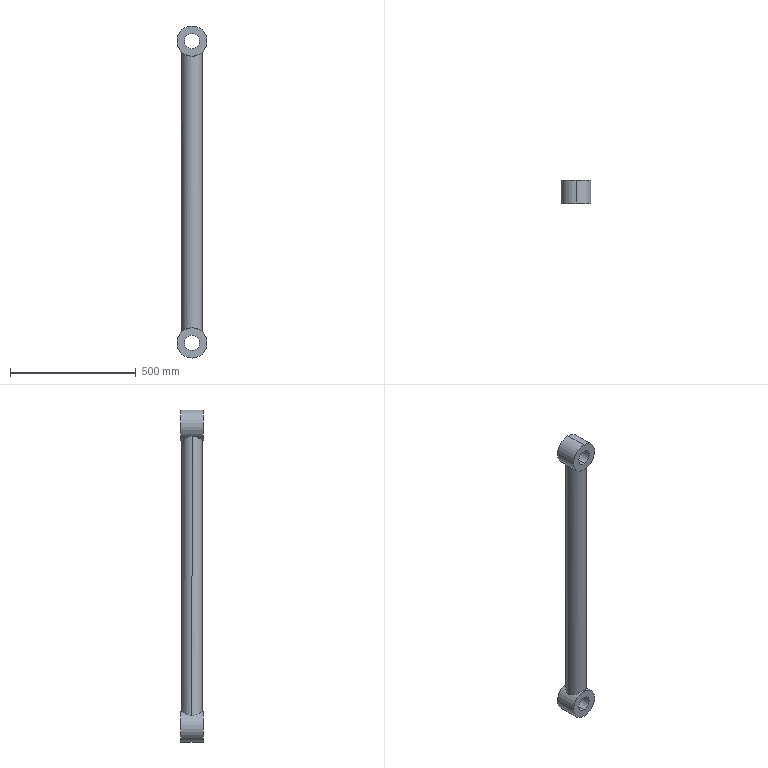Part | SolidWorks | features ICE 2, Extrusion 1, Scale 1 | 1 solid | 14 faces | box 120 x 90 x 1320 mm | volume 6991195 mm3 | cylinder 10 | plane 4 | commonest cylinder face diameters 60 x4 120 x4 80 x2
STEP:
#1=CARTESIAN_POINT('',(0.000008321,45.,-630.));
#2=VERTEX_POINT('',#1);
#3=CARTESIAN_POINT('',(0.000008321,45.,-570.));
#4=VERTEX_POINT('',#3);
#5=CARTESIAN_POINT('',(0.000008321,45.,-600.));
#6=DIRECTION('',(0.,1.,0.));
#7=DIRECTION('',(0.,0.,-1.));
#8=AXIS2_PLACEMENT_3D('',#5,#6,#7);
#9=CIRCLE('',#8,30.);
#10=EDGE_CURVE('',#2,#4,#9,.T.);
#11=ORIENTED_EDGE('',*,*,#10,.T.);
#12=CARTESIAN_POINT('',(0.000008321,-45.,-570.));
#13=VERTEX_POINT('',#12);
#14=CARTESIAN_POINT('',(0.000008321,45.,-570.));
#15=DIRECTION('',(0.,-1.,0.));
#16=VECTOR('',#15,1000.);
#17=LINE('',#14,#16);
#18=EDGE_CURVE('',#4,#13,#17,.T.);
#19=ORIENTED_EDGE('',*,*,#18,.T.);
#20=CARTESIAN_POINT('',(0.000008321,-45.,-630.));
#21=VERTEX_POINT('',#20);
#22=CARTESIAN_POINT('',(0.000008321,-45.,-600.));
#23=DIRECTION('',(0.,1.,0.));
#24=DIRECTION('',(0.,0.,-1.));
#25=AXIS2_PLACEMENT_3D('',#22,#23,#24);
#26=CIRCLE('',#25,30.);
#27=EDGE_CURVE('',#21,#13,#26,.T.);
#28=ORIENTED_EDGE('',*,*,#27,.F.);
#29=CARTESIAN_POINT('',(0.000008321,45.,-630.));
#30=DIRECTION('',(0.,-1.,0.));
#31=VECTOR('',#30,1000.);
#32=LINE('',#29,#31);
#33=EDGE_CURVE('',#2,#21,#32,.T.);
#34=ORIENTED_EDGE('',*,*,#33,.F.);
#35=EDGE_LOOP('',(#11,#19,#28,#34));
#36=FACE_OUTER_BOUND('',#35,.T.);
#37=CARTESIAN_POINT('',(0.000008321,45.,-600.));
#38=DIRECTION('',(0.,-1.,0.));
#39=DIRECTION('',(0.,0.,-1.));
#40=AXIS2_PLACEMENT_3D('',#37,#38,#39);
#41=CYLINDRICAL_SURFACE('',#40,30.);
#42=ADVANCED_FACE('',(#36),#41,.F.);
#43=CARTESIAN_POINT('',(0.000008321,45.,-540.));
#44=VERTEX_POINT('',#43);
#45=CARTESIAN_POINT('',(0.000008321,45.,-660.));
#46=VERTEX_POINT('',#45);
#47=CARTESIAN_POINT('',(0.000008321,45.,-600.));
#48=DIRECTION('',(0.,1.,0.));
#49=DIRECTION('',(0.,0.,-1.));
#50=AXIS2_PLACEMENT_3D('',#47,#48,#49);
#51=CIRCLE('',#50,60.);
#52=EDGE_CURVE('',#44,#46,#51,.T.);
#53=ORIENTED_EDGE('',*,*,#52,.F.);
#54=CARTESIAN_POINT('',(0.000008321,40.,-540.));
#55=VERTEX_POINT('',#54);
#56=CARTESIAN_POINT('',(0.000008321,45.,-540.));
#57=DIRECTION('',(0.,-1.,0.));
#58=VECTOR('',#57,1000.);
#59=LINE('',#56,#58);
#60=EDGE_CURVE('',#44,#55,#59,.T.);
#61=ORIENTED_EDGE('',*,*,#60,.T.);
#62=CARTESIAN_POINT('',(40.,0.00004525,-555.278));
#63=VERTEX_POINT('',#62);
#64=CARTESIAN_POINT('',(0.000008321,40.,-540.));
#65=CARTESIAN_POINT('',(0.6813,40.,-540.));
#66=CARTESIAN_POINT('',(1.367,39.982,-540.011));
#67=CARTESIAN_POINT('',(2.725,39.913,-540.058));
#68=CARTESIAN_POINT('',(3.4,39.861,-540.092));
#69=CARTESIAN_POINT('',(5.412,39.655,-540.229));
#70=CARTESIAN_POINT('',(6.739,39.451,-540.365));
#71=CARTESIAN_POINT('',(9.361,38.912,-540.72));
#72=CARTESIAN_POINT('',(10.656,38.578,-540.939));
#73=CARTESIAN_POINT('',(13.218,37.777,-541.459));
#74=CARTESIAN_POINT('',(14.462,37.317,-541.755));
#75=CARTESIAN_POINT('',(16.878,36.288,-542.409));
#76=CARTESIAN_POINT('',(18.051,35.719,-542.767));
#77=CARTESIAN_POINT('',(19.76,34.785,-543.344));
#78=CARTESIAN_POINT('',(20.321,34.46,-543.543));
#79=CARTESIAN_POINT('',(21.427,33.783,-543.953));
#80=CARTESIAN_POINT('',(21.973,33.431,-544.165));
#81=CARTESIAN_POINT('',(24.644,31.612,-545.246));
#82=CARTESIAN_POINT('',(26.594,29.986,-546.177));
#83=CARTESIAN_POINT('',(29.268,27.294,-547.613));
#84=CARTESIAN_POINT('',(30.118,26.354,-548.098));
#85=CARTESIAN_POINT('',(31.734,24.383,-549.07));
#86=CARTESIAN_POINT('',(32.492,23.363,-549.552));
#87=CARTESIAN_POINT('',(34.611,20.211,-550.959));
#88=CARTESIAN_POINT('',(35.824,17.982,-551.851));
#89=CARTESIAN_POINT('',(37.085,15.003,-552.832));
#90=CARTESIAN_POINT('',(37.325,14.398,-553.022));
#91=CARTESIAN_POINT('',(37.777,13.166,-553.384));
#92=CARTESIAN_POINT('',(37.99,12.538,-553.558));
#93=CARTESIAN_POINT('',(38.581,10.642,-554.046));
#94=CARTESIAN_POINT('',(38.913,9.359,-554.328));
#95=CARTESIAN_POINT('',(39.449,6.75,-554.79));
#96=CARTESIAN_POINT('',(39.653,5.426,-554.97));
#97=CARTESIAN_POINT('',(39.861,3.405,-555.154));
#98=CARTESIAN_POINT('',(39.913,2.723,-555.201));
#99=CARTESIAN_POINT('',(39.983,1.358,-555.263));
#100=CARTESIAN_POINT('',(40.,0.6779,-555.278));
#101=CARTESIAN_POINT('',(40.,0.00004525,-555.278));
#102=B_SPLINE_CURVE_WITH_KNOTS('',3,(#64,#65,#66,#67,#68,#69,#70,#71,#72,#73,#74,#75,#76,#77,#78,#79,#80,#81,#82,#83,#84,#85,#86,#87,#88,#89,#90,#91,#92,#93,#94,#95,#96,#97,#98,#99,#100,#101),.UNSPECIFIED.,.F.,.F.,(4,2,2,2,2,2,2,2,2,2,2,2,2,2,2,2,2,2,4),(0.0647,0.06672,0.06873,0.07276,0.07679,0.08082,0.08485,0.08687,0.08889,0.09695,0.101,0.105,0.1131,0.1151,0.1171,0.1211,0.1252,0.1272,0.1292),.UNSPECIFIED.);
#103=EDGE_CURVE('',#55,#63,#102,.T.);
#104=ORIENTED_EDGE('',*,*,#103,.T.);
#105=CARTESIAN_POINT('',(0.000008321,-40.,-540.));
#106=VERTEX_POINT('',#105);
#107=CARTESIAN_POINT('',(40.,0.00004525,-555.278));
#108=CARTESIAN_POINT('',(40.,-2.71,-555.278));
#109=CARTESIAN_POINT('',(39.728,-5.383,-555.031));
#110=CARTESIAN_POINT('',(39.052,-8.681,-554.448));
#111=CARTESIAN_POINT('',(38.901,-9.335,-554.319));
#112=CARTESIAN_POINT('',(38.569,-10.624,-554.038));
#113=CARTESIAN_POINT('',(38.388,-11.26,-553.887));
#114=CARTESIAN_POINT('',(37.801,-13.145,-553.402));
#115=CARTESIAN_POINT('',(37.352,-14.371,-553.04));
#116=CARTESIAN_POINT('',(36.34,-16.766,-552.252));
#117=CARTESIAN_POINT('',(35.775,-17.94,-551.826));
#118=CARTESIAN_POINT('',(34.549,-20.2,-550.939));
#119=CARTESIAN_POINT('',(33.888,-21.29,-550.478));
#120=CARTESIAN_POINT('',(32.47,-23.394,-549.538));
#121=CARTESIAN_POINT('',(31.714,-24.41,-549.057));
#122=CARTESIAN_POINT('',(30.506,-25.88,-548.332));
#123=CARTESIAN_POINT('',(30.091,-26.361,-548.089));
#124=CARTESIAN_POINT('',(29.236,-27.306,-547.602));
#125=CARTESIAN_POINT('',(28.797,-27.769,-547.36));
#126=CARTESIAN_POINT('',(26.556,-30.021,-546.158));
#127=CARTESIAN_POINT('',(24.609,-31.638,-545.231));
#128=CARTESIAN_POINT('',(21.438,-33.794,-543.949));
#129=CARTESIAN_POINT('',(20.339,-34.467,-543.539));
#130=CARTESIAN_POINT('',(18.623,-35.407,-542.96));
#131=CARTESIAN_POINT('',(18.037,-35.709,-542.772));
#132=CARTESIAN_POINT('',(16.853,-36.282,-542.412));
#133=CARTESIAN_POINT('',(16.254,-36.554,-542.24));
#134=CARTESIAN_POINT('',(13.228,-37.841,-541.422));
#135=CARTESIAN_POINT('',(10.701,-38.637,-540.901));
#136=CARTESIAN_POINT('',(7.394,-39.316,-540.453));
#137=CARTESIAN_POINT('',(6.722,-39.437,-540.374));
#138=CARTESIAN_POINT('',(5.381,-39.642,-540.238));
#139=CARTESIAN_POINT('',(4.709,-39.728,-540.181));
#140=CARTESIAN_POINT('',(2.694,-39.932,-540.045));
#141=CARTESIAN_POINT('',(1.348,-40.,-540.));
#142=CARTESIAN_POINT('',(0.000008321,-40.,-540.));
#143=B_SPLINE_CURVE_WITH_KNOTS('',3,(#107,#108,#109,#110,#111,#112,#113,#114,#115,#116,#117,#118,#119,#120,#121,#122,#123,#124,#125,#126,#127,#128,#129,#130,#131,#132,#133,#134,#135,#136,#137,#138,#139,#140,#141,#142),.UNSPECIFIED.,.F.,.F.,(4,2,2,2,2,2,2,2,2,2,2,2,2,2,2,2,2,4),(0.1292,0.1372,0.1393,0.1413,0.1453,0.1493,0.1534,0.1574,0.1594,0.1614,0.1695,0.1735,0.1755,0.1775,0.1856,0.1876,0.1896,0.1936),.UNSPECIFIED.);
#144=EDGE_CURVE('',#63,#106,#143,.T.);
#145=ORIENTED_EDGE('',*,*,#144,.T.);
#146=CARTESIAN_POINT('',(0.000008321,-45.,-540.));
#147=VERTEX_POINT('',#146);
#148=CARTESIAN_POINT('',(0.000008321,45.,-540.));
#149=DIRECTION('',(0.,-1.,0.));
#150=VECTOR('',#149,1000.);
#151=LINE('',#148,#150);
#152=EDGE_CURVE('',#106,#147,#151,.T.);
#153=ORIENTED_EDGE('',*,*,#152,.T.);
#154=CARTESIAN_POINT('',(0.000008321,-45.,-660.));
#155=VERTEX_POINT('',#154);
#156=CARTESIAN_POINT('',(0.000008321,-45.,-600.));
#157=DIRECTION('',(0.,1.,0.));
#158=DIRECTION('',(0.,0.,-1.));
#159=AXIS2_PLACEMENT_3D('',#156,#157,#158);
#160=CIRCLE('',#159,60.);
#161=EDGE_CURVE('',#147,#155,#160,.T.);
#162=ORIENTED_EDGE('',*,*,#161,.T.);
#163=CARTESIAN_POINT('',(0.000008321,45.,-660.));
#164=DIRECTION('',(0.,-1.,0.));
#165=VECTOR('',#164,1000.);
#166=LINE('',#163,#165);
#167=EDGE_CURVE('',#46,#155,#166,.T.);
#168=ORIENTED_EDGE('',*,*,#167,.F.);
#169=EDGE_LOOP('',(#53,#61,#104,#145,#153,#162,#168));
#170=FACE_OUTER_BOUND('',#169,.T.);
#171=CARTESIAN_POINT('',(0.000008321,45.,-600.));
#172=DIRECTION('',(0.,-1.,0.));
#173=DIRECTION('',(0.,0.,-1.));
#174=AXIS2_PLACEMENT_3D('',#171,#172,#173);
#175=CYLINDRICAL_SURFACE('',#174,60.);
#176=ADVANCED_FACE('',(#170),#175,.T.);
#177=CARTESIAN_POINT('',(0.000008321,45.,570.));
#178=VERTEX_POINT('',#177);
#179=CARTESIAN_POINT('',(0.000008321,45.,630.));
#180=VERTEX_POINT('',#179);
#181=CARTESIAN_POINT('',(0.000008321,45.,600.));
#182=DIRECTION('',(0.,1.,0.));
#183=DIRECTION('',(0.,0.,1.));
#184=AXIS2_PLACEMENT_3D('',#181,#182,#183);
#185=CIRCLE('',#184,30.);
#186=EDGE_CURVE('',#178,#180,#185,.T.);
#187=ORIENTED_EDGE('',*,*,#186,.T.);
#188=CARTESIAN_POINT('',(0.000008321,-45.,630.));
#189=VERTEX_POINT('',#188);
#190=CARTESIAN_POINT('',(0.000008321,45.,630.));
#191=DIRECTION('',(0.,-1.,0.));
#192=VECTOR('',#191,1000.);
#193=LINE('',#190,#192);
#194=EDGE_CURVE('',#180,#189,#193,.T.);
#195=ORIENTED_EDGE('',*,*,#194,.T.);
#196=CARTESIAN_POINT('',(0.000008321,-45.,570.));
#197=VERTEX_POINT('',#196);
#198=CARTESIAN_POINT('',(0.000008321,-45.,600.));
#199=DIRECTION('',(0.,1.,0.));
#200=DIRECTION('',(0.,0.,1.));
#201=AXIS2_PLACEMENT_3D('',#198,#199,#200);
#202=CIRCLE('',#201,30.);
#203=EDGE_CURVE('',#197,#189,#202,.T.);
#204=ORIENTED_EDGE('',*,*,#203,.F.);
#205=CARTESIAN_POINT('',(0.000008321,45.,570.));
#206=DIRECTION('',(0.,-1.,0.));
#207=VECTOR('',#206,1000.);
#208=LINE('',#205,#207);
#209=EDGE_CURVE('',#178,#197,#208,.T.);
#210=ORIENTED_EDGE('',*,*,#209,.F.);
#211=EDGE_LOOP('',(#187,#195,#204,#210));
#212=FACE_OUTER_BOUND('',#211,.T.);
#213=CARTESIAN_POINT('',(0.000008321,45.,600.));
#214=DIRECTION('',(0.,-1.,0.));
#215=DIRECTION('',(0.,0.,-1.));
#216=AXIS2_PLACEMENT_3D('',#213,#214,#215);
#217=CYLINDRICAL_SURFACE('',#216,30.);
#218=ADVANCED_FACE('',(#212),#217,.F.);
#219=CARTESIAN_POINT('',(0.000008321,45.,660.));
#220=VERTEX_POINT('',#219);
#221=CARTESIAN_POINT('',(0.000008321,45.,540.));
#222=VERTEX_POINT('',#221);
#223=CARTESIAN_POINT('',(0.000008321,45.,600.));
#224=DIRECTION('',(0.,1.,0.));
#225=DIRECTION('',(0.,0.,1.));
#226=AXIS2_PLACEMENT_3D('',#223,#224,#225);
#227=CIRCLE('',#226,60.);
#228=EDGE_CURVE('',#220,#222,#227,.T.);
#229=ORIENTED_EDGE('',*,*,#228,.F.);
#230=CARTESIAN_POINT('',(0.000008321,-45.,660.));
#231=VERTEX_POINT('',#230);
#232=CARTESIAN_POINT('',(0.000008321,45.,660.));
#233=DIRECTION('',(0.,-1.,0.));
#234=VECTOR('',#233,1000.);
#235=LINE('',#232,#234);
#236=EDGE_CURVE('',#220,#231,#235,.T.);
#237=ORIENTED_EDGE('',*,*,#236,.T.);
#238=CARTESIAN_POINT('',(0.000008321,-45.,540.));
#239=VERTEX_POINT('',#238);
#240=CARTESIAN_POINT('',(0.000008321,-45.,600.));
#241=DIRECTION('',(0.,1.,0.));
#242=DIRECTION('',(0.,0.,1.));
#243=AXIS2_PLACEMENT_3D('',#240,#241,#242);
#244=CIRCLE('',#243,60.);
#245=EDGE_CURVE('',#231,#239,#244,.T.);
#246=ORIENTED_EDGE('',*,*,#245,.T.);
#247=CARTESIAN_POINT('',(0.000008321,-40.,540.));
#248=VERTEX_POINT('',#247);
#249=CARTESIAN_POINT('',(0.000008321,45.,540.));
#250=DIRECTION('',(0.,-1.,0.));
#251=VECTOR('',#250,1000.);
#252=LINE('',#249,#251);
#253=EDGE_CURVE('',#248,#239,#252,.T.);
#254=ORIENTED_EDGE('',*,*,#253,.F.);
#255=CARTESIAN_POINT('',(40.,0.00004525,555.279));
#256=VERTEX_POINT('',#255);
#257=CARTESIAN_POINT('',(0.000008321,-40.,540.));
#258=CARTESIAN_POINT('',(0.6813,-40.,540.));
#259=CARTESIAN_POINT('',(1.367,-39.982,540.012));
#260=CARTESIAN_POINT('',(2.725,-39.913,540.058));
#261=CARTESIAN_POINT('',(3.4,-39.861,540.093));
#262=CARTESIAN_POINT('',(5.412,-39.655,540.23));
#263=CARTESIAN_POINT('',(6.739,-39.451,540.365));
#264=CARTESIAN_POINT('',(9.361,-38.912,540.72));
#265=CARTESIAN_POINT('',(10.656,-38.578,540.94));
#266=CARTESIAN_POINT('',(13.218,-37.777,541.46));
#267=CARTESIAN_POINT('',(14.462,-37.317,541.756));
#268=CARTESIAN_POINT('',(16.878,-36.288,542.41));
#269=CARTESIAN_POINT('',(18.051,-35.719,542.767));
#270=CARTESIAN_POINT('',(19.76,-34.785,543.344));
#271=CARTESIAN_POINT('',(20.321,-34.46,543.543));
#272=CARTESIAN_POINT('',(21.427,-33.783,543.953));
#273=CARTESIAN_POINT('',(21.973,-33.431,544.165));
#274=CARTESIAN_POINT('',(24.644,-31.612,545.247));
#275=CARTESIAN_POINT('',(26.594,-29.986,546.178));
#276=CARTESIAN_POINT('',(29.268,-27.294,547.613));
#277=CARTESIAN_POINT('',(30.118,-26.354,548.099));
#278=CARTESIAN_POINT('',(31.734,-24.383,549.071));
#279=CARTESIAN_POINT('',(32.492,-23.363,549.553));
#280=CARTESIAN_POINT('',(34.611,-20.211,550.96));
#281=CARTESIAN_POINT('',(35.824,-17.982,551.852));
#282=CARTESIAN_POINT('',(37.085,-15.003,552.833));
#283=CARTESIAN_POINT('',(37.325,-14.398,553.022));
#284=CARTESIAN_POINT('',(37.777,-13.166,553.385));
#285=CARTESIAN_POINT('',(37.99,-12.538,553.559));
#286=CARTESIAN_POINT('',(38.581,-10.642,554.046));
#287=CARTESIAN_POINT('',(38.913,-9.358,554.328));
#288=CARTESIAN_POINT('',(39.449,-6.75,554.791));
#289=CARTESIAN_POINT('',(39.653,-5.426,554.971));
#290=CARTESIAN_POINT('',(39.861,-3.404,555.155));
#291=CARTESIAN_POINT('',(39.913,-2.723,555.201));
#292=CARTESIAN_POINT('',(39.983,-1.358,555.263));
#293=CARTESIAN_POINT('',(40.,-0.6778,555.279));
#294=CARTESIAN_POINT('',(40.,0.00004525,555.279));
#295=B_SPLINE_CURVE_WITH_KNOTS('',3,(#257,#258,#259,#260,#261,#262,#263,#264,#265,#266,#267,#268,#269,#270,#271,#272,#273,#274,#275,#276,#277,#278,#279,#280,#281,#282,#283,#284,#285,#286,#287,#288,#289,#290,#291,#292,#293,#294),.UNSPECIFIED.,.F.,.F.,(4,2,2,2,2,2,2,2,2,2,2,2,2,2,2,2,2,2,4),(0.0647,0.06672,0.06873,0.07276,0.07679,0.08082,0.08485,0.08687,0.08889,0.09695,0.101,0.105,0.1131,0.1151,0.1171,0.1211,0.1252,0.1272,0.1292),.UNSPECIFIED.);
#296=EDGE_CURVE('',#248,#256,#295,.T.);
#297=ORIENTED_EDGE('',*,*,#296,.T.);
#298=CARTESIAN_POINT('',(0.000008321,40.,540.));
#299=VERTEX_POINT('',#298);
#300=CARTESIAN_POINT('',(40.,0.00004525,555.279));
#301=CARTESIAN_POINT('',(40.,2.71,555.279));
#302=CARTESIAN_POINT('',(39.728,5.383,555.031));
#303=CARTESIAN_POINT('',(39.052,8.681,554.449));
#304=CARTESIAN_POINT('',(38.901,9.335,554.319));
#305=CARTESIAN_POINT('',(38.569,10.624,554.039));
#306=CARTESIAN_POINT('',(38.388,11.26,553.887));
#307=CARTESIAN_POINT('',(37.801,13.145,553.403));
#308=CARTESIAN_POINT('',(37.352,14.371,553.04));
#309=CARTESIAN_POINT('',(36.34,16.766,552.253));
#310=CARTESIAN_POINT('',(35.775,17.94,551.826));
#311=CARTESIAN_POINT('',(34.549,20.2,550.939));
#312=CARTESIAN_POINT('',(33.888,21.29,550.479));
#313=CARTESIAN_POINT('',(32.47,23.395,549.538));
#314=CARTESIAN_POINT('',(31.714,24.41,549.058));
#315=CARTESIAN_POINT('',(30.506,25.88,548.332));
#316=CARTESIAN_POINT('',(30.091,26.361,548.089));
#317=CARTESIAN_POINT('',(29.236,27.306,547.603));
#318=CARTESIAN_POINT('',(28.797,27.769,547.36));
#319=CARTESIAN_POINT('',(26.556,30.021,546.159));
#320=CARTESIAN_POINT('',(24.609,31.638,545.232));
#321=CARTESIAN_POINT('',(21.438,33.794,543.949));
#322=CARTESIAN_POINT('',(20.339,34.468,543.54));
#323=CARTESIAN_POINT('',(18.623,35.407,542.96));
#324=CARTESIAN_POINT('',(18.037,35.709,542.772));
#325=CARTESIAN_POINT('',(16.853,36.282,542.412));
#326=CARTESIAN_POINT('',(16.254,36.554,542.241));
#327=CARTESIAN_POINT('',(13.228,37.841,541.423));
#328=CARTESIAN_POINT('',(10.701,38.637,540.902));
#329=CARTESIAN_POINT('',(7.394,39.317,540.454));
#330=CARTESIAN_POINT('',(6.722,39.437,540.374));
#331=CARTESIAN_POINT('',(5.381,39.642,540.238));
#332=CARTESIAN_POINT('',(4.709,39.728,540.182));
#333=CARTESIAN_POINT('',(2.694,39.932,540.046));
#334=CARTESIAN_POINT('',(1.348,40.,540.));
#335=CARTESIAN_POINT('',(0.000008321,40.,540.));
#336=B_SPLINE_CURVE_WITH_KNOTS('',3,(#300,#301,#302,#303,#304,#305,#306,#307,#308,#309,#310,#311,#312,#313,#314,#315,#316,#317,#318,#319,#320,#321,#322,#323,#324,#325,#326,#327,#328,#329,#330,#331,#332,#333,#334,#335),.UNSPECIFIED.,.F.,.F.,(4,2,2,2,2,2,2,2,2,2,2,2,2,2,2,2,2,4),(0.1292,0.1372,0.1393,0.1413,0.1453,0.1493,0.1534,0.1574,0.1594,0.1614,0.1695,0.1735,0.1755,0.1775,0.1856,0.1876,0.1896,0.1936),.UNSPECIFIED.);
#337=EDGE_CURVE('',#256,#299,#336,.T.);
#338=ORIENTED_EDGE('',*,*,#337,.T.);
#339=CARTESIAN_POINT('',(0.000008321,45.,540.));
#340=DIRECTION('',(0.,-1.,0.));
#341=VECTOR('',#340,1000.);
#342=LINE('',#339,#341);
#343=EDGE_CURVE('',#222,#299,#342,.T.);
#344=ORIENTED_EDGE('',*,*,#343,.F.);
#345=EDGE_LOOP('',(#229,#237,#246,#254,#297,#338,#344));
#346=FACE_OUTER_BOUND('',#345,.T.);
#347=CARTESIAN_POINT('',(0.000008321,45.,600.));
#348=DIRECTION('',(0.,-1.,0.));
#349=DIRECTION('',(0.,0.,-1.));
#350=AXIS2_PLACEMENT_3D('',#347,#348,#349);
#351=CYLINDRICAL_SURFACE('',#350,60.);
#352=ADVANCED_FACE('',(#346),#351,.T.);
#353=ORIENTED_EDGE('',*,*,#337,.F.);
#354=CARTESIAN_POINT('',(40.,0.00004525,600.));
#355=DIRECTION('',(0.,0.,-1.));
#356=VECTOR('',#355,1000.);
#357=LINE('',#354,#356);
#358=EDGE_CURVE('',#256,#63,#357,.T.);
#359=ORIENTED_EDGE('',*,*,#358,.T.);
#360=ORIENTED_EDGE('',*,*,#103,.F.);
#361=CARTESIAN_POINT('',(-40.,0.00004525,-555.278));
#362=VERTEX_POINT('',#361);
#363=CARTESIAN_POINT('',(-40.,0.00004525,-555.278));
#364=CARTESIAN_POINT('',(-40.,2.746,-555.278));
#365=CARTESIAN_POINT('',(-39.721,5.418,-555.025));
#366=CARTESIAN_POINT('',(-39.053,8.68,-554.448));
#367=CARTESIAN_POINT('',(-38.903,9.329,-554.32));
#368=CARTESIAN_POINT('',(-38.571,10.617,-554.04));
#369=CARTESIAN_POINT('',(-38.388,11.26,-553.887));
#370=CARTESIAN_POINT('',(-37.796,13.162,-553.398));
#371=CARTESIAN_POINT('',(-37.344,14.39,-553.034));
#372=CARTESIAN_POINT('',(-36.334,16.779,-552.248));
#373=CARTESIAN_POINT('',(-35.775,17.939,-551.826));
#374=CARTESIAN_POINT('',(-34.857,19.632,-551.162));
#375=CARTESIAN_POINT('',(-34.538,20.188,-550.935));
#376=CARTESIAN_POINT('',(-33.872,21.286,-550.474));
#377=CARTESIAN_POINT('',(-33.526,21.827,-550.238));
#378=CARTESIAN_POINT('',(-31.74,24.477,-549.053));
#379=CARTESIAN_POINT('',(-30.135,26.426,-548.076));
#380=CARTESIAN_POINT('',(-27.452,29.12,-546.639));
#381=CARTESIAN_POINT('',(-26.512,29.98,-546.164));
#382=CARTESIAN_POINT('',(-24.532,31.62,-545.233));
#383=CARTESIAN_POINT('',(-23.506,32.39,-544.784));
#384=CARTESIAN_POINT('',(-20.325,34.546,-543.501));
#385=CARTESIAN_POINT('',(-18.066,35.784,-542.73));
#386=CARTESIAN_POINT('',(-15.047,37.068,-541.914));
#387=CARTESIAN_POINT('',(-14.433,37.311,-541.758));
#388=CARTESIAN_POINT('',(-13.185,37.77,-541.463));
#389=CARTESIAN_POINT('',(-12.548,37.987,-541.323));
#390=CARTESIAN_POINT('',(-10.628,38.586,-540.934));
#391=CARTESIAN_POINT('',(-9.333,38.919,-540.715));
#392=CARTESIAN_POINT('',(-5.407,39.723,-540.186));
#393=CARTESIAN_POINT('',(-2.734,40.,-540.));
#394=CARTESIAN_POINT('',(0.000008321,40.,-540.));
#395=B_SPLINE_CURVE_WITH_KNOTS('',3,(#363,#364,#365,#366,#367,#368,#369,#370,#371,#372,#373,#374,#375,#376,#377,#378,#379,#380,#381,#382,#383,#384,#385,#386,#387,#388,#389,#390,#391,#392,#393,#394),.UNSPECIFIED.,.F.,.F.,(4,2,2,2,2,2,2,2,2,2,2,2,2,2,2,4),(0.,0.008088,0.01011,0.01213,0.01618,0.02022,0.02224,0.02426,0.03235,0.03639,0.04044,0.04853,0.05055,0.05257,0.05661,0.0647),.UNSPECIFIED.);
#396=EDGE_CURVE('',#362,#55,#395,.T.);
#397=ORIENTED_EDGE('',*,*,#396,.F.);
#398=CARTESIAN_POINT('',(-40.,0.00004525,555.279));
#399=VERTEX_POINT('',#398);
#400=CARTESIAN_POINT('',(-40.,0.00004525,600.));
#401=DIRECTION('',(0.,0.,-1.));
#402=VECTOR('',#401,1000.);
#403=LINE('',#400,#402);
#404=EDGE_CURVE('',#399,#362,#403,.T.);
#405=ORIENTED_EDGE('',*,*,#404,.F.);
#406=CARTESIAN_POINT('',(0.000008321,40.,540.));
#407=CARTESIAN_POINT('',(-1.346,40.,540.));
#408=CARTESIAN_POINT('',(-2.694,39.932,540.046));
#409=CARTESIAN_POINT('',(-4.718,39.727,540.182));
#410=CARTESIAN_POINT('',(-5.396,39.64,540.24));
#411=CARTESIAN_POINT('',(-6.736,39.435,540.376));
#412=CARTESIAN_POINT('',(-7.4,39.315,540.455));
#413=CARTESIAN_POINT('',(-10.688,38.639,540.9));
#414=CARTESIAN_POINT('',(-13.218,37.846,541.42));
#415=CARTESIAN_POINT('',(-16.265,36.55,542.244));
#416=CARTESIAN_POINT('',(-16.866,36.276,542.416));
#417=CARTESIAN_POINT('',(-18.046,35.704,542.775));
#418=CARTESIAN_POINT('',(-18.625,35.405,542.961));
#419=CARTESIAN_POINT('',(-20.333,34.471,543.538));
#420=CARTESIAN_POINT('',(-21.431,33.799,543.947));
#421=CARTESIAN_POINT('',(-23.553,32.356,544.805));
#422=CARTESIAN_POINT('',(-24.577,31.585,545.254));
#423=CARTESIAN_POINT('',(-26.551,29.945,546.184));
#424=CARTESIAN_POINT('',(-27.489,29.086,546.658));
#425=CARTESIAN_POINT('',(-30.162,26.394,548.093));
#426=CARTESIAN_POINT('',(-31.761,24.449,549.067));
#427=CARTESIAN_POINT('',(-33.894,21.279,550.483));
#428=CARTESIAN_POINT('',(-34.562,20.178,550.949));
#429=CARTESIAN_POINT('',(-35.782,17.924,551.832));
#430=CARTESIAN_POINT('',(-36.339,16.768,552.252));
#431=CARTESIAN_POINT('',(-37.344,14.39,553.034));
#432=CARTESIAN_POINT('',(-37.793,13.169,553.396));
#433=CARTESIAN_POINT('',(-38.381,11.284,553.881));
#434=CARTESIAN_POINT('',(-38.563,10.646,554.034));
#435=CARTESIAN_POINT('',(-38.897,9.351,554.316));
#436=CARTESIAN_POINT('',(-39.049,8.698,554.446));
#437=CARTESIAN_POINT('',(-39.452,6.73,554.794));
#438=CARTESIAN_POINT('',(-39.656,5.405,554.973));
#439=CARTESIAN_POINT('',(-39.861,3.395,555.155));
#440=CARTESIAN_POINT('',(-39.913,2.721,555.201));
#441=CARTESIAN_POINT('',(-39.965,1.705,555.248));
#442=CARTESIAN_POINT('',(-39.978,1.365,555.259));
#443=CARTESIAN_POINT('',(-39.996,0.6841,555.275));
#444=CARTESIAN_POINT('',(-40.,0.3414,555.279));
#445=CARTESIAN_POINT('',(-40.,0.00004525,555.279));
#446=B_SPLINE_CURVE_WITH_KNOTS('',3,(#406,#407,#408,#409,#410,#411,#412,#413,#414,#415,#416,#417,#418,#419,#420,#421,#422,#423,#424,#425,#426,#427,#428,#429,#430,#431,#432,#433,#434,#435,#436,#437,#438,#439,#440,#441,#442,#443,#444,#445),.UNSPECIFIED.,.F.,.F.,(4,2,2,2,2,2,2,2,2,2,2,2,2,2,2,2,2,2,2,4),(0.1936,0.1977,0.1997,0.2017,0.2097,0.2117,0.2138,0.2178,0.2218,0.2258,0.2339,0.2379,0.2419,0.2459,0.2479,0.25,0.254,0.256,0.257,0.258),.UNSPECIFIED.);
#447=EDGE_CURVE('',#299,#399,#446,.T.);
#448=ORIENTED_EDGE('',*,*,#447,.F.);
#449=EDGE_LOOP('',(#353,#359,#360,#397,#405,#448));
#450=FACE_OUTER_BOUND('',#449,.T.);
#451=CARTESIAN_POINT('',(0.000008321,0.00004525,600.));
#452=DIRECTION('',(0.,0.,-1.));
#453=DIRECTION('',(-1.,0.,0.));
#454=AXIS2_PLACEMENT_3D('',#451,#452,#453);
#455=CYLINDRICAL_SURFACE('',#454,40.);
#456=ADVANCED_FACE('',(#450),#455,.T.);
#457=ORIENTED_EDGE('',*,*,#358,.F.);
#458=ORIENTED_EDGE('',*,*,#296,.F.);
#459=CARTESIAN_POINT('',(-40.,0.00004525,555.279));
#460=CARTESIAN_POINT('',(-40.,-2.746,555.279));
#461=CARTESIAN_POINT('',(-39.721,-5.418,555.025));
#462=CARTESIAN_POINT('',(-39.053,-8.68,554.449));
#463=CARTESIAN_POINT('',(-38.903,-9.328,554.321));
#464=CARTESIAN_POINT('',(-38.571,-10.617,554.04));
#465=CARTESIAN_POINT('',(-38.388,-11.26,553.887));
#466=CARTESIAN_POINT('',(-37.796,-13.162,553.398));
#467=CARTESIAN_POINT('',(-37.344,-14.39,553.034));
#468=CARTESIAN_POINT('',(-36.334,-16.779,552.248));
#469=CARTESIAN_POINT('',(-35.775,-17.939,551.826));
#470=CARTESIAN_POINT('',(-34.857,-19.632,551.162));
#471=CARTESIAN_POINT('',(-34.538,-20.188,550.936));
#472=CARTESIAN_POINT('',(-33.872,-21.285,550.474));
#473=CARTESIAN_POINT('',(-33.526,-21.827,550.239));
#474=CARTESIAN_POINT('',(-31.74,-24.477,549.054));
#475=CARTESIAN_POINT('',(-30.135,-26.426,548.077));
#476=CARTESIAN_POINT('',(-27.452,-29.12,546.639));
#477=CARTESIAN_POINT('',(-26.512,-29.98,546.164));
#478=CARTESIAN_POINT('',(-24.532,-31.62,545.234));
#479=CARTESIAN_POINT('',(-23.506,-32.39,544.784));
#480=CARTESIAN_POINT('',(-20.325,-34.546,543.501));
#481=CARTESIAN_POINT('',(-18.066,-35.784,542.73));
#482=CARTESIAN_POINT('',(-15.047,-37.068,541.914));
#483=CARTESIAN_POINT('',(-14.433,-37.311,541.759));
#484=CARTESIAN_POINT('',(-13.185,-37.77,541.463));
#485=CARTESIAN_POINT('',(-12.548,-37.987,541.323));
#486=CARTESIAN_POINT('',(-10.628,-38.586,540.935));
#487=CARTESIAN_POINT('',(-9.333,-38.919,540.716));
#488=CARTESIAN_POINT('',(-5.407,-39.723,540.186));
#489=CARTESIAN_POINT('',(-2.734,-40.,540.));
#490=CARTESIAN_POINT('',(0.000008321,-40.,540.));
#491=B_SPLINE_CURVE_WITH_KNOTS('',3,(#459,#460,#461,#462,#463,#464,#465,#466,#467,#468,#469,#470,#471,#472,#473,#474,#475,#476,#477,#478,#479,#480,#481,#482,#483,#484,#485,#486,#487,#488,#489,#490),.UNSPECIFIED.,.F.,.F.,(4,2,2,2,2,2,2,2,2,2,2,2,2,2,2,4),(0.,0.008088,0.01011,0.01213,0.01618,0.02022,0.02224,0.02426,0.03235,0.03639,0.04044,0.04853,0.05055,0.05257,0.05661,0.0647),.UNSPECIFIED.);
#492=EDGE_CURVE('',#399,#248,#491,.T.);
#493=ORIENTED_EDGE('',*,*,#492,.F.);
#494=ORIENTED_EDGE('',*,*,#404,.T.);
#495=CARTESIAN_POINT('',(0.000008321,-40.,-540.));
#496=CARTESIAN_POINT('',(-1.346,-40.,-540.));
#497=CARTESIAN_POINT('',(-2.694,-39.932,-540.045));
#498=CARTESIAN_POINT('',(-4.718,-39.726,-540.182));
#499=CARTESIAN_POINT('',(-5.396,-39.64,-540.239));
#500=CARTESIAN_POINT('',(-6.736,-39.434,-540.375));
#501=CARTESIAN_POINT('',(-7.4,-39.315,-540.454));
#502=CARTESIAN_POINT('',(-10.688,-38.639,-540.9));
#503=CARTESIAN_POINT('',(-13.218,-37.846,-541.419));
#504=CARTESIAN_POINT('',(-16.265,-36.55,-542.243));
#505=CARTESIAN_POINT('',(-16.866,-36.276,-542.416));
#506=CARTESIAN_POINT('',(-18.046,-35.704,-542.774));
#507=CARTESIAN_POINT('',(-18.625,-35.405,-542.961));
#508=CARTESIAN_POINT('',(-20.333,-34.471,-543.537));
#509=CARTESIAN_POINT('',(-21.431,-33.799,-543.946));
#510=CARTESIAN_POINT('',(-23.553,-32.356,-544.804));
#511=CARTESIAN_POINT('',(-24.577,-31.585,-545.253));
#512=CARTESIAN_POINT('',(-26.551,-29.945,-546.183));
#513=CARTESIAN_POINT('',(-27.489,-29.085,-546.658));
#514=CARTESIAN_POINT('',(-30.162,-26.394,-548.093));
#515=CARTESIAN_POINT('',(-31.761,-24.449,-549.067));
#516=CARTESIAN_POINT('',(-33.894,-21.279,-550.483));
#517=CARTESIAN_POINT('',(-34.562,-20.178,-550.948));
#518=CARTESIAN_POINT('',(-35.782,-17.924,-551.831));
#519=CARTESIAN_POINT('',(-36.339,-16.767,-552.252));
#520=CARTESIAN_POINT('',(-37.344,-14.39,-553.034));
#521=CARTESIAN_POINT('',(-37.793,-13.169,-553.395));
#522=CARTESIAN_POINT('',(-38.381,-11.284,-553.881));
#523=CARTESIAN_POINT('',(-38.563,-10.646,-554.033));
#524=CARTESIAN_POINT('',(-38.897,-9.351,-554.316));
#525=CARTESIAN_POINT('',(-39.049,-8.697,-554.445));
#526=CARTESIAN_POINT('',(-39.452,-6.73,-554.793));
#527=CARTESIAN_POINT('',(-39.656,-5.405,-554.973));
#528=CARTESIAN_POINT('',(-39.861,-3.395,-555.155));
#529=CARTESIAN_POINT('',(-39.913,-2.721,-555.201));
#530=CARTESIAN_POINT('',(-39.965,-1.705,-555.247));
#531=CARTESIAN_POINT('',(-39.978,-1.365,-555.259));
#532=CARTESIAN_POINT('',(-39.996,-0.684,-555.274));
#533=CARTESIAN_POINT('',(-40.,-0.3413,-555.278));
#534=CARTESIAN_POINT('',(-40.,0.00004525,-555.278));
#535=B_SPLINE_CURVE_WITH_KNOTS('',3,(#495,#496,#497,#498,#499,#500,#501,#502,#503,#504,#505,#506,#507,#508,#509,#510,#511,#512,#513,#514,#515,#516,#517,#518,#519,#520,#521,#522,#523,#524,#525,#526,#527,#528,#529,#530,#531,#532,#533,#534),.UNSPECIFIED.,.F.,.F.,(4,2,2,2,2,2,2,2,2,2,2,2,2,2,2,2,2,2,2,4),(0.1936,0.1977,0.1997,0.2017,0.2097,0.2117,0.2138,0.2178,0.2218,0.2258,0.2339,0.2379,0.2419,0.2459,0.2479,0.25,0.254,0.256,0.257,0.258),.UNSPECIFIED.);
#536=EDGE_CURVE('',#106,#362,#535,.T.);
#537=ORIENTED_EDGE('',*,*,#536,.F.);
#538=ORIENTED_EDGE('',*,*,#144,.F.);
#539=EDGE_LOOP('',(#457,#458,#493,#494,#537,#538));
#540=FACE_OUTER_BOUND('',#539,.T.);
#541=CARTESIAN_POINT('',(0.000008321,0.00004525,600.));
#542=DIRECTION('',(0.,0.,-1.));
#543=DIRECTION('',(-1.,0.,0.));
#544=AXIS2_PLACEMENT_3D('',#541,#542,#543);
#545=CYLINDRICAL_SURFACE('',#544,40.);
#546=ADVANCED_FACE('',(#540),#545,.T.);
#547=ORIENTED_EDGE('',*,*,#236,.F.);
#548=CARTESIAN_POINT('',(0.000008321,45.,600.));
#549=DIRECTION('',(0.,1.,0.));
#550=DIRECTION('',(0.,0.,1.));
#551=AXIS2_PLACEMENT_3D('',#548,#549,#550);
#552=CIRCLE('',#551,60.);
#553=EDGE_CURVE('',#222,#220,#552,.T.);
#554=ORIENTED_EDGE('',*,*,#553,.F.);
#555=ORIENTED_EDGE('',*,*,#343,.T.);
#556=ORIENTED_EDGE('',*,*,#447,.T.);
#557=ORIENTED_EDGE('',*,*,#492,.T.);
#558=ORIENTED_EDGE('',*,*,#253,.T.);
#559=CARTESIAN_POINT('',(0.000008321,-45.,600.));
#560=DIRECTION('',(0.,1.,0.));
#561=DIRECTION('',(0.,0.,1.));
#562=AXIS2_PLACEMENT_3D('',#559,#560,#561);
#563=CIRCLE('',#562,60.);
#564=EDGE_CURVE('',#239,#231,#563,.T.);
#565=ORIENTED_EDGE('',*,*,#564,.T.);
#566=EDGE_LOOP('',(#547,#554,#555,#556,#557,#558,#565));
#567=FACE_OUTER_BOUND('',#566,.T.);
#568=CARTESIAN_POINT('',(0.000008321,45.,600.));
#569=DIRECTION('',(0.,-1.,0.));
#570=DIRECTION('',(0.,0.,-1.));
#571=AXIS2_PLACEMENT_3D('',#568,#569,#570);
#572=CYLINDRICAL_SURFACE('',#571,60.);
#573=ADVANCED_FACE('',(#567),#572,.T.);
#574=ORIENTED_EDGE('',*,*,#553,.T.);
#575=ORIENTED_EDGE('',*,*,#228,.T.);
#576=EDGE_LOOP('',(#574,#575));
#577=FACE_OUTER_BOUND('',#576,.T.);
#578=ORIENTED_EDGE('',*,*,#186,.F.);
#579=CARTESIAN_POINT('',(0.000008321,45.,600.));
#580=DIRECTION('',(0.,1.,0.));
#581=DIRECTION('',(0.,0.,1.));
#582=AXIS2_PLACEMENT_3D('',#579,#580,#581);
#583=CIRCLE('',#582,30.);
#584=EDGE_CURVE('',#180,#178,#583,.T.);
#585=ORIENTED_EDGE('',*,*,#584,.F.);
#586=EDGE_LOOP('',(#578,#585));
#587=FACE_BOUND('',#586,.T.);
#588=CARTESIAN_POINT('',(0.000008321,45.,600.));
#589=DIRECTION('',(0.,1.,0.));
#590=DIRECTION('',(0.,0.,1.));
#591=AXIS2_PLACEMENT_3D('',#588,#589,#590);
#592=PLANE('',#591);
#593=ADVANCED_FACE('',(#577,#587),#592,.T.);
#594=ORIENTED_EDGE('',*,*,#564,.F.);
#595=ORIENTED_EDGE('',*,*,#245,.F.);
#596=EDGE_LOOP('',(#594,#595));
#597=FACE_OUTER_BOUND('',#596,.T.);
#598=ORIENTED_EDGE('',*,*,#203,.T.);
#599=CARTESIAN_POINT('',(0.000008321,-45.,600.));
#600=DIRECTION('',(0.,1.,0.));
#601=DIRECTION('',(0.,0.,1.));
#602=AXIS2_PLACEMENT_3D('',#599,#600,#601);
#603=CIRCLE('',#602,30.);
#604=EDGE_CURVE('',#189,#197,#603,.T.);
#605=ORIENTED_EDGE('',*,*,#604,.T.);
#606=EDGE_LOOP('',(#598,#605));
#607=FACE_BOUND('',#606,.T.);
#608=CARTESIAN_POINT('',(0.000008321,-45.,600.));
#609=DIRECTION('',(0.,1.,0.));
#610=DIRECTION('',(0.,0.,1.));
#611=AXIS2_PLACEMENT_3D('',#608,#609,#610);
#612=PLANE('',#611);
#613=ADVANCED_FACE('',(#597,#607),#612,.F.);
#614=ORIENTED_EDGE('',*,*,#194,.F.);
#615=ORIENTED_EDGE('',*,*,#584,.T.);
#616=ORIENTED_EDGE('',*,*,#209,.T.);
#617=ORIENTED_EDGE('',*,*,#604,.F.);
#618=EDGE_LOOP('',(#614,#615,#616,#617));
#619=FACE_OUTER_BOUND('',#618,.T.);
#620=CARTESIAN_POINT('',(0.000008321,45.,600.));
#621=DIRECTION('',(0.,-1.,0.));
#622=DIRECTION('',(0.,0.,-1.));
#623=AXIS2_PLACEMENT_3D('',#620,#621,#622);
#624=CYLINDRICAL_SURFACE('',#623,30.);
#625=ADVANCED_FACE('',(#619),#624,.F.);
#626=ORIENTED_EDGE('',*,*,#60,.F.);
#627=CARTESIAN_POINT('',(0.000008321,45.,-600.));
#628=DIRECTION('',(0.,1.,0.));
#629=DIRECTION('',(0.,0.,-1.));
#630=AXIS2_PLACEMENT_3D('',#627,#628,#629);
#631=CIRCLE('',#630,60.);
#632=EDGE_CURVE('',#46,#44,#631,.T.);
#633=ORIENTED_EDGE('',*,*,#632,.F.);
#634=ORIENTED_EDGE('',*,*,#167,.T.);
#635=CARTESIAN_POINT('',(0.000008321,-45.,-600.));
#636=DIRECTION('',(0.,1.,0.));
#637=DIRECTION('',(0.,0.,-1.));
#638=AXIS2_PLACEMENT_3D('',#635,#636,#637);
#639=CIRCLE('',#638,60.);
#640=EDGE_CURVE('',#155,#147,#639,.T.);
#641=ORIENTED_EDGE('',*,*,#640,.T.);
#642=ORIENTED_EDGE('',*,*,#152,.F.);
#643=ORIENTED_EDGE('',*,*,#536,.T.);
#644=ORIENTED_EDGE('',*,*,#396,.T.);
#645=EDGE_LOOP('',(#626,#633,#634,#641,#642,#643,#644));
#646=FACE_OUTER_BOUND('',#645,.T.);
#647=CARTESIAN_POINT('',(0.000008321,45.,-600.));
#648=DIRECTION('',(0.,-1.,0.));
#649=DIRECTION('',(0.,0.,-1.));
#650=AXIS2_PLACEMENT_3D('',#647,#648,#649);
#651=CYLINDRICAL_SURFACE('',#650,60.);
#652=ADVANCED_FACE('',(#646),#651,.T.);
#653=ORIENTED_EDGE('',*,*,#18,.F.);
#654=CARTESIAN_POINT('',(0.000008321,45.,-600.));
#655=DIRECTION('',(0.,1.,0.));
#656=DIRECTION('',(0.,0.,-1.));
#657=AXIS2_PLACEMENT_3D('',#654,#655,#656);
#658=CIRCLE('',#657,30.);
#659=EDGE_CURVE('',#4,#2,#658,.T.);
#660=ORIENTED_EDGE('',*,*,#659,.T.);
#661=ORIENTED_EDGE('',*,*,#33,.T.);
#662=CARTESIAN_POINT('',(0.000008321,-45.,-600.));
#663=DIRECTION('',(0.,1.,0.));
#664=DIRECTION('',(0.,0.,-1.));
#665=AXIS2_PLACEMENT_3D('',#662,#663,#664);
#666=CIRCLE('',#665,30.);
#667=EDGE_CURVE('',#13,#21,#666,.T.);
#668=ORIENTED_EDGE('',*,*,#667,.F.);
#669=EDGE_LOOP('',(#653,#660,#661,#668));
#670=FACE_OUTER_BOUND('',#669,.T.);
#671=CARTESIAN_POINT('',(0.000008321,45.,-600.));
#672=DIRECTION('',(0.,-1.,0.));
#673=DIRECTION('',(0.,0.,-1.));
#674=AXIS2_PLACEMENT_3D('',#671,#672,#673);
#675=CYLINDRICAL_SURFACE('',#674,30.);
#676=ADVANCED_FACE('',(#670),#675,.F.);
#677=ORIENTED_EDGE('',*,*,#632,.T.);
#678=ORIENTED_EDGE('',*,*,#52,.T.);
#679=EDGE_LOOP('',(#677,#678));
#680=FACE_OUTER_BOUND('',#679,.T.);
#681=ORIENTED_EDGE('',*,*,#10,.F.);
#682=ORIENTED_EDGE('',*,*,#659,.F.);
#683=EDGE_LOOP('',(#681,#682));
#684=FACE_BOUND('',#683,.T.);
#685=CARTESIAN_POINT('',(0.000008321,45.,-600.));
#686=DIRECTION('',(0.,-1.,0.));
#687=DIRECTION('',(0.,0.,-1.));
#688=AXIS2_PLACEMENT_3D('',#685,#686,#687);
#689=PLANE('',#688);
#690=ADVANCED_FACE('',(#680,#684),#689,.F.);
#691=ORIENTED_EDGE('',*,*,#640,.F.);
#692=ORIENTED_EDGE('',*,*,#161,.F.);
#693=EDGE_LOOP('',(#691,#692));
#694=FACE_OUTER_BOUND('',#693,.T.);
#695=ORIENTED_EDGE('',*,*,#27,.T.);
#696=ORIENTED_EDGE('',*,*,#667,.T.);
#697=EDGE_LOOP('',(#695,#696));
#698=FACE_BOUND('',#697,.T.);
#699=CARTESIAN_POINT('',(0.000008321,-45.,-600.));
#700=DIRECTION('',(0.,-1.,0.));
#701=DIRECTION('',(0.,0.,-1.));
#702=AXIS2_PLACEMENT_3D('',#699,#700,#701);
#703=PLANE('',#702);
#704=ADVANCED_FACE('',(#694,#698),#703,.T.);
#705=CLOSED_SHELL('',(#42,#176,#218,#352,#456,#546,#573,#593,#613,#625,#652,#676,#690,#704));
#706=MANIFOLD_SOLID_BREP('',#705);
#707=CARTESIAN_POINT('',(0.,0.,0.));
#708=DIRECTION('',(0.,0.,1.));
#709=DIRECTION('',(1.,0.,0.));
#710=AXIS2_PLACEMENT_3D('',#707,#708,#709);
#711=(LENGTH_UNIT()NAMED_UNIT(*)SI_UNIT(.MILLI.,.METRE.));
#712=UNCERTAINTY_MEASURE_WITH_UNIT(LENGTH_MEASURE(0.00001),#711,'','');
#713=(NAMED_UNIT(*)PLANE_ANGLE_UNIT()SI_UNIT($,.RADIAN.));
#714=(NAMED_UNIT(*)SI_UNIT($,.STERADIAN.)SOLID_ANGLE_UNIT());
#715=(GEOMETRIC_REPRESENTATION_CONTEXT(3)GLOBAL_UNCERTAINTY_ASSIGNED_CONTEXT((#712))GLOBAL_UNIT_ASSIGNED_CONTEXT((#711,#713,#714))REPRESENTATION_CONTEXT('',''));
#716=ADVANCED_BREP_SHAPE_REPRESENTATION('',(#706,#710),#715);